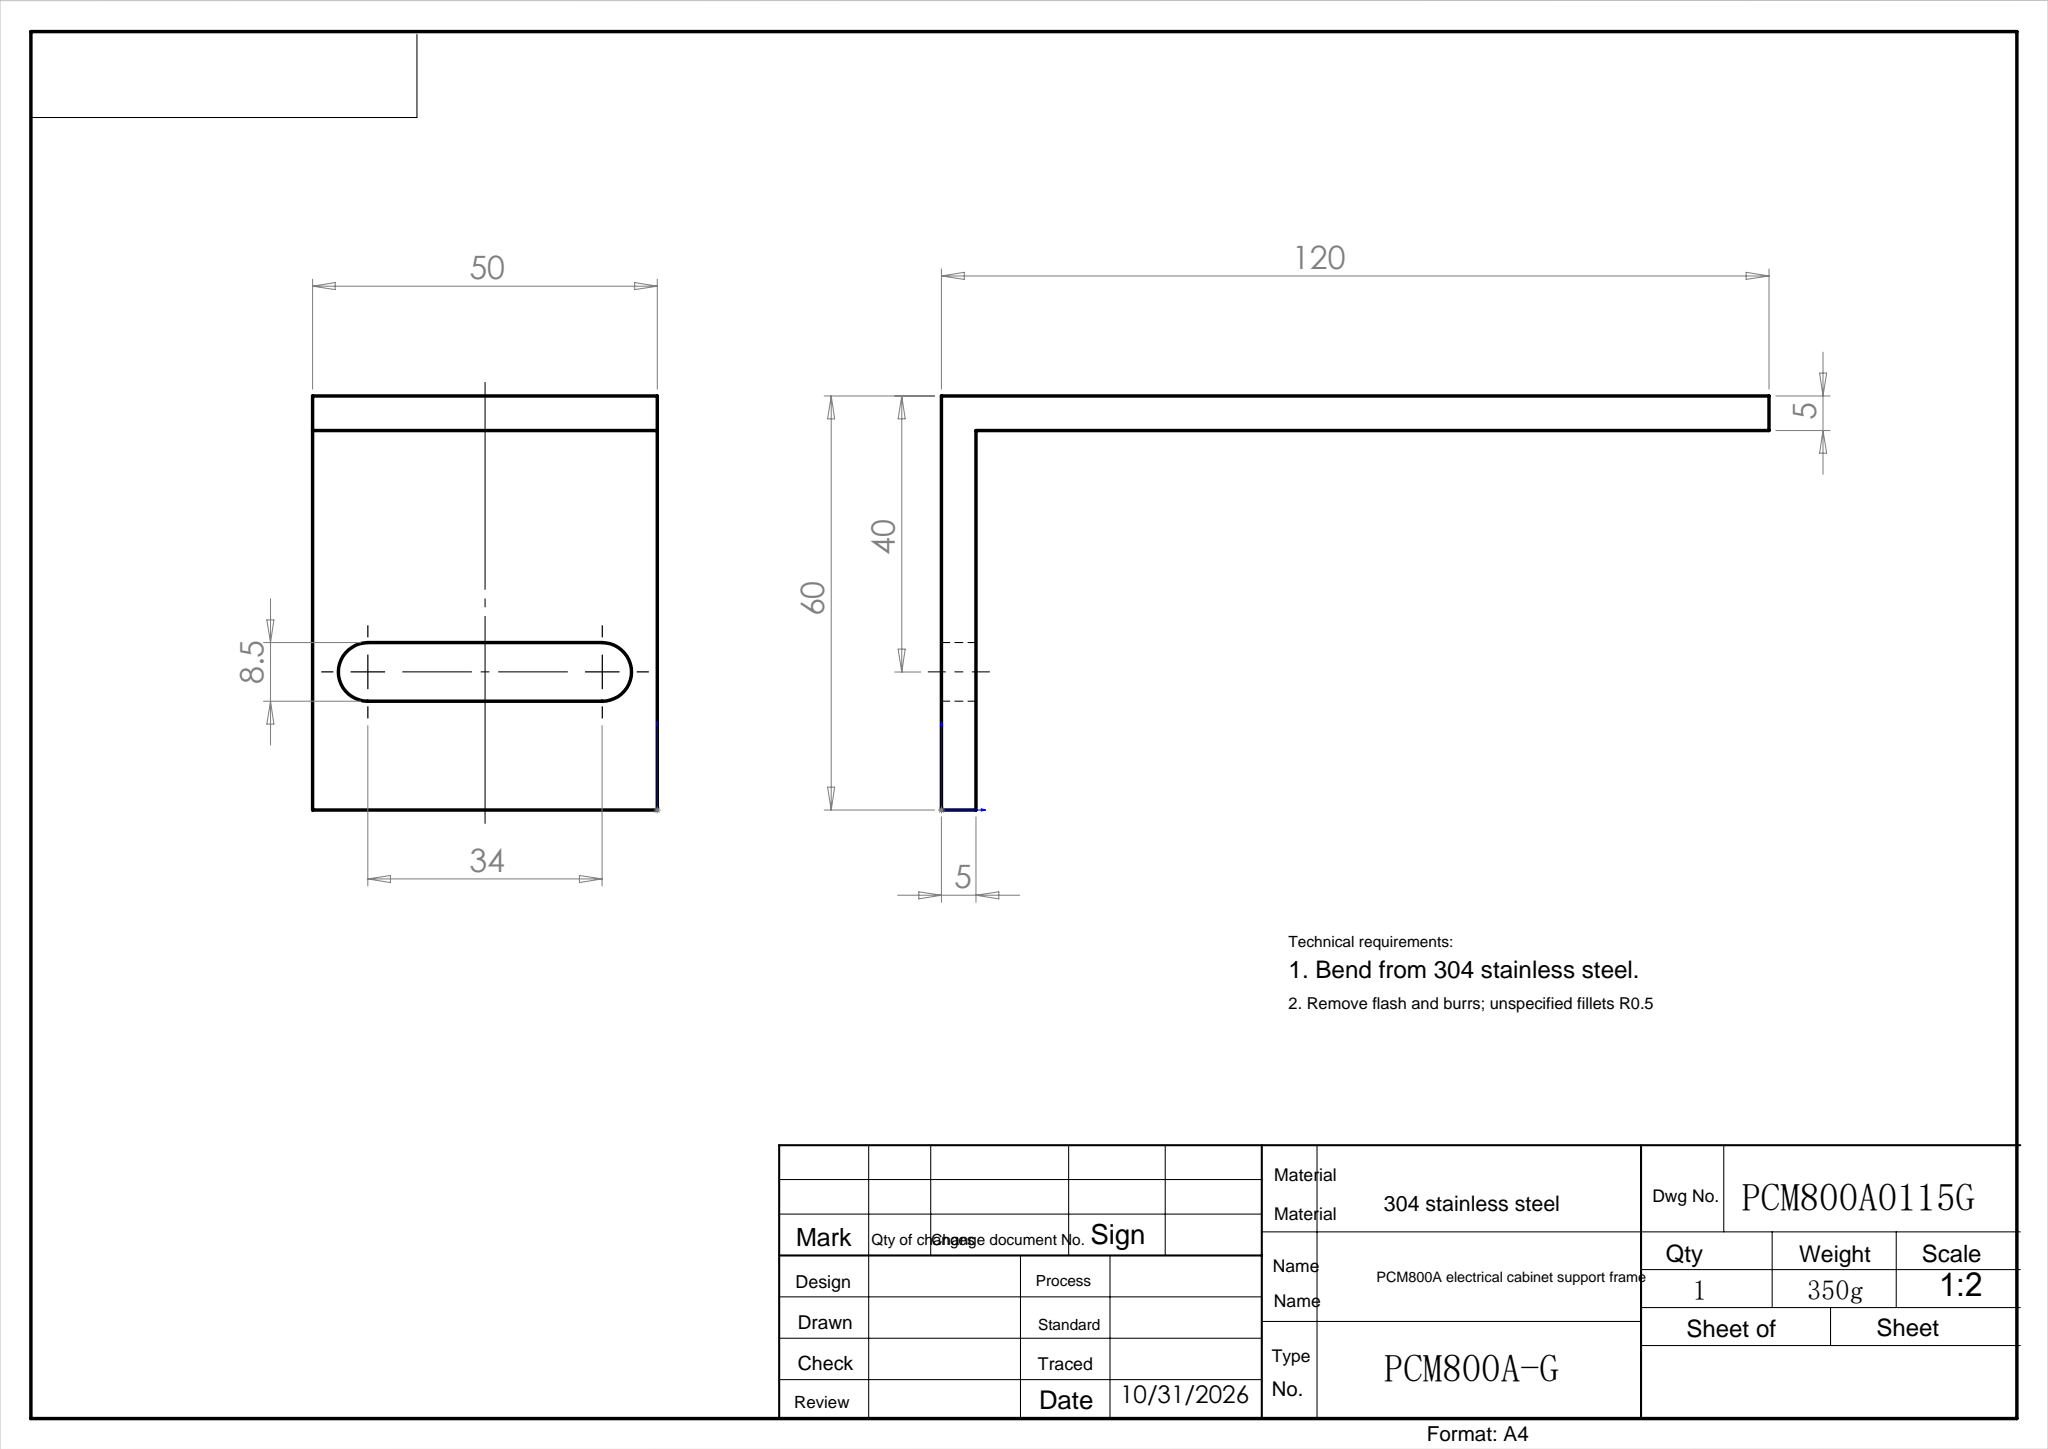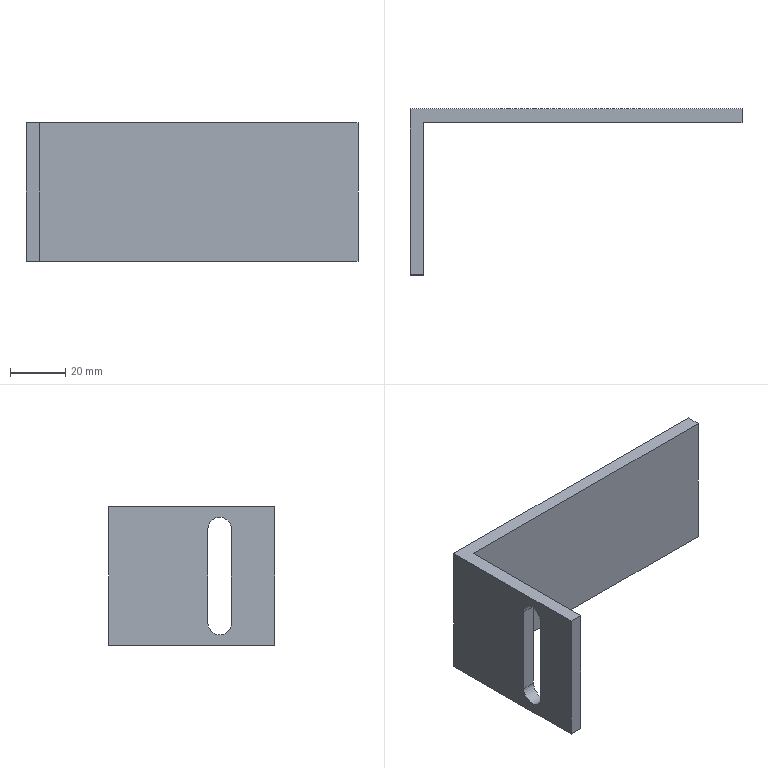Part | SolidWorks | features ExtruThin 1, ICE 1 | 1 solid | 13 faces | box 120 x 60 x 50 mm | volume 42021 mm3 | plane 10 | cylinder 3 | commonest cylinder face diameters 8.5 x3
STEP:
#1=CARTESIAN_POINT('',(5.,20.,46.25));
#2=VERTEX_POINT('',#1);
#3=CARTESIAN_POINT('',(5.,24.25,42.));
#4=VERTEX_POINT('',#3);
#5=CARTESIAN_POINT('',(5.,20.,42.));
#6=DIRECTION('',(-1.,0.,0.));
#7=DIRECTION('',(0.,0.,1.));
#8=AXIS2_PLACEMENT_3D('',#5,#6,#7);
#9=CIRCLE('',#8,4.25);
#10=EDGE_CURVE('',#2,#4,#9,.T.);
#11=ORIENTED_EDGE('',*,*,#10,.F.);
#12=CARTESIAN_POINT('',(0.,20.,46.25));
#13=VERTEX_POINT('',#12);
#14=CARTESIAN_POINT('',(10.,20.,46.25));
#15=DIRECTION('',(-1.,0.,0.));
#16=VECTOR('',#15,1000.);
#17=LINE('',#14,#16);
#18=EDGE_CURVE('',#2,#13,#17,.T.);
#19=ORIENTED_EDGE('',*,*,#18,.T.);
#20=CARTESIAN_POINT('',(0.,24.25,42.));
#21=VERTEX_POINT('',#20);
#22=CARTESIAN_POINT('',(0.,20.,42.));
#23=DIRECTION('',(-1.,0.,0.));
#24=DIRECTION('',(0.,0.,-1.));
#25=AXIS2_PLACEMENT_3D('',#22,#23,#24);
#26=CIRCLE('',#25,4.25);
#27=EDGE_CURVE('',#13,#21,#26,.T.);
#28=ORIENTED_EDGE('',*,*,#27,.T.);
#29=CARTESIAN_POINT('',(10.,24.25,42.));
#30=DIRECTION('',(-1.,0.,0.));
#31=VECTOR('',#30,1000.);
#32=LINE('',#29,#31);
#33=EDGE_CURVE('',#4,#21,#32,.T.);
#34=ORIENTED_EDGE('',*,*,#33,.F.);
#35=EDGE_LOOP('',(#11,#19,#28,#34));
#36=FACE_OUTER_BOUND('',#35,.T.);
#37=CARTESIAN_POINT('',(10.,20.,42.));
#38=DIRECTION('',(-1.,0.,0.));
#39=DIRECTION('',(0.,0.,1.));
#40=AXIS2_PLACEMENT_3D('',#37,#38,#39);
#41=CYLINDRICAL_SURFACE('',#40,4.25);
#42=ADVANCED_FACE('',(#36),#41,.F.);
#43=CARTESIAN_POINT('',(5.,55.,0.));
#44=VERTEX_POINT('',#43);
#45=CARTESIAN_POINT('',(120.,55.,0.));
#46=VERTEX_POINT('',#45);
#47=CARTESIAN_POINT('',(0.,55.,0.));
#48=DIRECTION('',(1.,0.,0.));
#49=VECTOR('',#48,1000.);
#50=LINE('',#47,#49);
#51=EDGE_CURVE('',#44,#46,#50,.T.);
#52=ORIENTED_EDGE('',*,*,#51,.T.);
#53=CARTESIAN_POINT('',(120.,55.,50.));
#54=VERTEX_POINT('',#53);
#55=CARTESIAN_POINT('',(120.,55.,50.));
#56=DIRECTION('',(0.,0.,-1.));
#57=VECTOR('',#56,1000.);
#58=LINE('',#55,#57);
#59=EDGE_CURVE('',#54,#46,#58,.T.);
#60=ORIENTED_EDGE('',*,*,#59,.F.);
#61=CARTESIAN_POINT('',(5.,55.,50.));
#62=VERTEX_POINT('',#61);
#63=CARTESIAN_POINT('',(0.,55.,50.));
#64=DIRECTION('',(1.,0.,0.));
#65=VECTOR('',#64,1000.);
#66=LINE('',#63,#65);
#67=EDGE_CURVE('',#62,#54,#66,.T.);
#68=ORIENTED_EDGE('',*,*,#67,.F.);
#69=CARTESIAN_POINT('',(5.,55.,50.));
#70=DIRECTION('',(0.,0.,-1.));
#71=VECTOR('',#70,1000.);
#72=LINE('',#69,#71);
#73=EDGE_CURVE('',#62,#44,#72,.T.);
#74=ORIENTED_EDGE('',*,*,#73,.T.);
#75=EDGE_LOOP('',(#52,#60,#68,#74));
#76=FACE_OUTER_BOUND('',#75,.T.);
#77=CARTESIAN_POINT('',(0.,55.,50.));
#78=DIRECTION('',(0.,1.,0.));
#79=DIRECTION('',(0.,0.,1.));
#80=AXIS2_PLACEMENT_3D('',#77,#78,#79);
#81=PLANE('',#80);
#82=ADVANCED_FACE('',(#76),#81,.F.);
#83=CARTESIAN_POINT('',(120.,60.,0.));
#84=VERTEX_POINT('',#83);
#85=CARTESIAN_POINT('',(120.,60.,0.));
#86=DIRECTION('',(0.,-1.,0.));
#87=VECTOR('',#86,1000.);
#88=LINE('',#85,#87);
#89=EDGE_CURVE('',#84,#46,#88,.T.);
#90=ORIENTED_EDGE('',*,*,#89,.F.);
#91=CARTESIAN_POINT('',(120.,60.,50.));
#92=VERTEX_POINT('',#91);
#93=CARTESIAN_POINT('',(120.,60.,50.));
#94=DIRECTION('',(0.,0.,-1.));
#95=VECTOR('',#94,1000.);
#96=LINE('',#93,#95);
#97=EDGE_CURVE('',#92,#84,#96,.T.);
#98=ORIENTED_EDGE('',*,*,#97,.F.);
#99=CARTESIAN_POINT('',(120.,60.,50.));
#100=DIRECTION('',(0.,-1.,0.));
#101=VECTOR('',#100,1000.);
#102=LINE('',#99,#101);
#103=EDGE_CURVE('',#92,#54,#102,.T.);
#104=ORIENTED_EDGE('',*,*,#103,.T.);
#105=ORIENTED_EDGE('',*,*,#59,.T.);
#106=EDGE_LOOP('',(#90,#98,#104,#105));
#107=FACE_OUTER_BOUND('',#106,.T.);
#108=CARTESIAN_POINT('',(120.,60.,50.));
#109=DIRECTION('',(1.,0.,0.));
#110=DIRECTION('',(0.,0.,-1.));
#111=AXIS2_PLACEMENT_3D('',#108,#109,#110);
#112=PLANE('',#111);
#113=ADVANCED_FACE('',(#107),#112,.T.);
#114=CARTESIAN_POINT('',(0.,60.,0.));
#115=VERTEX_POINT('',#114);
#116=CARTESIAN_POINT('',(0.,60.,0.));
#117=DIRECTION('',(1.,0.,0.));
#118=VECTOR('',#117,1000.);
#119=LINE('',#116,#118);
#120=EDGE_CURVE('',#115,#84,#119,.T.);
#121=ORIENTED_EDGE('',*,*,#120,.F.);
#122=CARTESIAN_POINT('',(0.,60.,50.));
#123=VERTEX_POINT('',#122);
#124=CARTESIAN_POINT('',(0.,60.,50.));
#125=DIRECTION('',(0.,0.,-1.));
#126=VECTOR('',#125,1000.);
#127=LINE('',#124,#126);
#128=EDGE_CURVE('',#123,#115,#127,.T.);
#129=ORIENTED_EDGE('',*,*,#128,.F.);
#130=CARTESIAN_POINT('',(0.,60.,50.));
#131=DIRECTION('',(1.,0.,0.));
#132=VECTOR('',#131,1000.);
#133=LINE('',#130,#132);
#134=EDGE_CURVE('',#123,#92,#133,.T.);
#135=ORIENTED_EDGE('',*,*,#134,.T.);
#136=ORIENTED_EDGE('',*,*,#97,.T.);
#137=EDGE_LOOP('',(#121,#129,#135,#136));
#138=FACE_OUTER_BOUND('',#137,.T.);
#139=CARTESIAN_POINT('',(0.,60.,50.));
#140=DIRECTION('',(0.,1.,0.));
#141=DIRECTION('',(0.,0.,1.));
#142=AXIS2_PLACEMENT_3D('',#139,#140,#141);
#143=PLANE('',#142);
#144=ADVANCED_FACE('',(#138),#143,.T.);
#145=CARTESIAN_POINT('',(0.,24.25,8.));
#146=VERTEX_POINT('',#145);
#147=CARTESIAN_POINT('',(0.,15.75,8.));
#148=VERTEX_POINT('',#147);
#149=CARTESIAN_POINT('',(0.,20.,8.));
#150=DIRECTION('',(-1.,0.,0.));
#151=DIRECTION('',(0.,0.,1.));
#152=AXIS2_PLACEMENT_3D('',#149,#150,#151);
#153=CIRCLE('',#152,4.25);
#154=EDGE_CURVE('',#146,#148,#153,.T.);
#155=ORIENTED_EDGE('',*,*,#154,.F.);
#156=CARTESIAN_POINT('',(0.,24.25,8.));
#157=DIRECTION('',(0.,0.,-1.));
#158=VECTOR('',#157,1000.);
#159=LINE('',#156,#158);
#160=EDGE_CURVE('',#21,#146,#159,.T.);
#161=ORIENTED_EDGE('',*,*,#160,.F.);
#162=ORIENTED_EDGE('',*,*,#27,.F.);
#163=CARTESIAN_POINT('',(0.,15.75,42.));
#164=VERTEX_POINT('',#163);
#165=CARTESIAN_POINT('',(0.,20.,42.));
#166=DIRECTION('',(-1.,0.,0.));
#167=DIRECTION('',(0.,0.,-1.));
#168=AXIS2_PLACEMENT_3D('',#165,#166,#167);
#169=CIRCLE('',#168,4.25);
#170=EDGE_CURVE('',#164,#13,#169,.T.);
#171=ORIENTED_EDGE('',*,*,#170,.F.);
#172=CARTESIAN_POINT('',(0.,15.75,8.));
#173=DIRECTION('',(0.,0.,1.));
#174=VECTOR('',#173,1000.);
#175=LINE('',#172,#174);
#176=EDGE_CURVE('',#148,#164,#175,.T.);
#177=ORIENTED_EDGE('',*,*,#176,.F.);
#178=EDGE_LOOP('',(#155,#161,#162,#171,#177));
#179=FACE_BOUND('',#178,.T.);
#180=CARTESIAN_POINT('',(0.,0.,0.));
#181=VERTEX_POINT('',#180);
#182=CARTESIAN_POINT('',(0.,0.,0.));
#183=DIRECTION('',(0.,1.,0.));
#184=VECTOR('',#183,1000.);
#185=LINE('',#182,#184);
#186=EDGE_CURVE('',#181,#115,#185,.T.);
#187=ORIENTED_EDGE('',*,*,#186,.F.);
#188=CARTESIAN_POINT('',(0.,0.,50.));
#189=VERTEX_POINT('',#188);
#190=CARTESIAN_POINT('',(0.,0.,50.));
#191=DIRECTION('',(0.,0.,-1.));
#192=VECTOR('',#191,1000.);
#193=LINE('',#190,#192);
#194=EDGE_CURVE('',#189,#181,#193,.T.);
#195=ORIENTED_EDGE('',*,*,#194,.F.);
#196=CARTESIAN_POINT('',(0.,0.,50.));
#197=DIRECTION('',(0.,1.,0.));
#198=VECTOR('',#197,1000.);
#199=LINE('',#196,#198);
#200=EDGE_CURVE('',#189,#123,#199,.T.);
#201=ORIENTED_EDGE('',*,*,#200,.T.);
#202=ORIENTED_EDGE('',*,*,#128,.T.);
#203=EDGE_LOOP('',(#187,#195,#201,#202));
#204=FACE_OUTER_BOUND('',#203,.T.);
#205=CARTESIAN_POINT('',(0.,0.,50.));
#206=DIRECTION('',(-1.,0.,0.));
#207=DIRECTION('',(0.,0.,1.));
#208=AXIS2_PLACEMENT_3D('',#205,#206,#207);
#209=PLANE('',#208);
#210=ADVANCED_FACE('',(#179,#204),#209,.T.);
#211=CARTESIAN_POINT('',(5.,0.,0.));
#212=VERTEX_POINT('',#211);
#213=CARTESIAN_POINT('',(5.,0.,0.));
#214=DIRECTION('',(-1.,0.,0.));
#215=VECTOR('',#214,1000.);
#216=LINE('',#213,#215);
#217=EDGE_CURVE('',#212,#181,#216,.T.);
#218=ORIENTED_EDGE('',*,*,#217,.F.);
#219=CARTESIAN_POINT('',(5.,0.,50.));
#220=VERTEX_POINT('',#219);
#221=CARTESIAN_POINT('',(5.,0.,50.));
#222=DIRECTION('',(0.,0.,-1.));
#223=VECTOR('',#222,1000.);
#224=LINE('',#221,#223);
#225=EDGE_CURVE('',#220,#212,#224,.T.);
#226=ORIENTED_EDGE('',*,*,#225,.F.);
#227=CARTESIAN_POINT('',(5.,0.,50.));
#228=DIRECTION('',(-1.,0.,0.));
#229=VECTOR('',#228,1000.);
#230=LINE('',#227,#229);
#231=EDGE_CURVE('',#220,#189,#230,.T.);
#232=ORIENTED_EDGE('',*,*,#231,.T.);
#233=ORIENTED_EDGE('',*,*,#194,.T.);
#234=EDGE_LOOP('',(#218,#226,#232,#233));
#235=FACE_OUTER_BOUND('',#234,.T.);
#236=CARTESIAN_POINT('',(5.,0.,50.));
#237=DIRECTION('',(0.,-1.,0.));
#238=DIRECTION('',(0.,0.,-1.));
#239=AXIS2_PLACEMENT_3D('',#236,#237,#238);
#240=PLANE('',#239);
#241=ADVANCED_FACE('',(#235),#240,.T.);
#242=CARTESIAN_POINT('',(5.,24.25,8.));
#243=VERTEX_POINT('',#242);
#244=CARTESIAN_POINT('',(5.,24.25,50.));
#245=DIRECTION('',(0.,0.,-1.));
#246=VECTOR('',#245,1000.);
#247=LINE('',#244,#246);
#248=EDGE_CURVE('',#4,#243,#247,.T.);
#249=ORIENTED_EDGE('',*,*,#248,.T.);
#250=CARTESIAN_POINT('',(5.,15.75,8.));
#251=VERTEX_POINT('',#250);
#252=CARTESIAN_POINT('',(5.,20.,8.));
#253=DIRECTION('',(-1.,0.,0.));
#254=DIRECTION('',(0.,0.,1.));
#255=AXIS2_PLACEMENT_3D('',#252,#253,#254);
#256=CIRCLE('',#255,4.25);
#257=EDGE_CURVE('',#243,#251,#256,.T.);
#258=ORIENTED_EDGE('',*,*,#257,.T.);
#259=CARTESIAN_POINT('',(5.,15.75,42.));
#260=VERTEX_POINT('',#259);
#261=CARTESIAN_POINT('',(5.,15.75,50.));
#262=DIRECTION('',(0.,0.,1.));
#263=VECTOR('',#262,1000.);
#264=LINE('',#261,#263);
#265=EDGE_CURVE('',#251,#260,#264,.T.);
#266=ORIENTED_EDGE('',*,*,#265,.T.);
#267=CARTESIAN_POINT('',(5.,20.,42.));
#268=DIRECTION('',(-1.,0.,0.));
#269=DIRECTION('',(0.,0.,1.));
#270=AXIS2_PLACEMENT_3D('',#267,#268,#269);
#271=CIRCLE('',#270,4.25);
#272=EDGE_CURVE('',#260,#2,#271,.T.);
#273=ORIENTED_EDGE('',*,*,#272,.T.);
#274=ORIENTED_EDGE('',*,*,#10,.T.);
#275=EDGE_LOOP('',(#249,#258,#266,#273,#274));
#276=FACE_BOUND('',#275,.T.);
#277=CARTESIAN_POINT('',(5.,0.,0.));
#278=DIRECTION('',(0.,1.,0.));
#279=VECTOR('',#278,1000.);
#280=LINE('',#277,#279);
#281=EDGE_CURVE('',#212,#44,#280,.T.);
#282=ORIENTED_EDGE('',*,*,#281,.T.);
#283=ORIENTED_EDGE('',*,*,#73,.F.);
#284=CARTESIAN_POINT('',(5.,0.,50.));
#285=DIRECTION('',(0.,1.,0.));
#286=VECTOR('',#285,1000.);
#287=LINE('',#284,#286);
#288=EDGE_CURVE('',#220,#62,#287,.T.);
#289=ORIENTED_EDGE('',*,*,#288,.F.);
#290=ORIENTED_EDGE('',*,*,#225,.T.);
#291=EDGE_LOOP('',(#282,#283,#289,#290));
#292=FACE_OUTER_BOUND('',#291,.T.);
#293=CARTESIAN_POINT('',(5.,0.,50.));
#294=DIRECTION('',(-1.,0.,0.));
#295=DIRECTION('',(0.,0.,1.));
#296=AXIS2_PLACEMENT_3D('',#293,#294,#295);
#297=PLANE('',#296);
#298=ADVANCED_FACE('',(#276,#292),#297,.F.);
#299=ORIENTED_EDGE('',*,*,#67,.T.);
#300=ORIENTED_EDGE('',*,*,#103,.F.);
#301=ORIENTED_EDGE('',*,*,#134,.F.);
#302=ORIENTED_EDGE('',*,*,#200,.F.);
#303=ORIENTED_EDGE('',*,*,#231,.F.);
#304=ORIENTED_EDGE('',*,*,#288,.T.);
#305=EDGE_LOOP('',(#299,#300,#301,#302,#303,#304));
#306=FACE_OUTER_BOUND('',#305,.T.);
#307=CARTESIAN_POINT('',(120.,55.,50.));
#308=DIRECTION('',(0.,0.,-1.));
#309=DIRECTION('',(-1.,0.,0.));
#310=AXIS2_PLACEMENT_3D('',#307,#308,#309);
#311=PLANE('',#310);
#312=ADVANCED_FACE('',(#306),#311,.F.);
#313=ORIENTED_EDGE('',*,*,#51,.F.);
#314=ORIENTED_EDGE('',*,*,#281,.F.);
#315=ORIENTED_EDGE('',*,*,#217,.T.);
#316=ORIENTED_EDGE('',*,*,#186,.T.);
#317=ORIENTED_EDGE('',*,*,#120,.T.);
#318=ORIENTED_EDGE('',*,*,#89,.T.);
#319=EDGE_LOOP('',(#313,#314,#315,#316,#317,#318));
#320=FACE_OUTER_BOUND('',#319,.T.);
#321=CARTESIAN_POINT('',(120.,55.,0.));
#322=DIRECTION('',(0.,0.,-1.));
#323=DIRECTION('',(-1.,0.,0.));
#324=AXIS2_PLACEMENT_3D('',#321,#322,#323);
#325=PLANE('',#324);
#326=ADVANCED_FACE('',(#320),#325,.T.);
#327=CARTESIAN_POINT('',(10.,24.25,8.));
#328=DIRECTION('',(-1.,0.,0.));
#329=VECTOR('',#328,1000.);
#330=LINE('',#327,#329);
#331=EDGE_CURVE('',#243,#146,#330,.T.);
#332=ORIENTED_EDGE('',*,*,#331,.T.);
#333=ORIENTED_EDGE('',*,*,#154,.T.);
#334=CARTESIAN_POINT('',(10.,15.75,8.));
#335=DIRECTION('',(-1.,0.,0.));
#336=VECTOR('',#335,1000.);
#337=LINE('',#334,#336);
#338=EDGE_CURVE('',#251,#148,#337,.T.);
#339=ORIENTED_EDGE('',*,*,#338,.F.);
#340=ORIENTED_EDGE('',*,*,#257,.F.);
#341=EDGE_LOOP('',(#332,#333,#339,#340));
#342=FACE_OUTER_BOUND('',#341,.T.);
#343=CARTESIAN_POINT('',(10.,20.,8.));
#344=DIRECTION('',(-1.,0.,0.));
#345=DIRECTION('',(0.,0.,1.));
#346=AXIS2_PLACEMENT_3D('',#343,#344,#345);
#347=CYLINDRICAL_SURFACE('',#346,4.25);
#348=ADVANCED_FACE('',(#342),#347,.F.);
#349=ORIENTED_EDGE('',*,*,#33,.T.);
#350=ORIENTED_EDGE('',*,*,#160,.T.);
#351=ORIENTED_EDGE('',*,*,#331,.F.);
#352=ORIENTED_EDGE('',*,*,#248,.F.);
#353=EDGE_LOOP('',(#349,#350,#351,#352));
#354=FACE_OUTER_BOUND('',#353,.T.);
#355=CARTESIAN_POINT('',(10.,24.25,8.));
#356=DIRECTION('',(0.,1.,0.));
#357=DIRECTION('',(0.,0.,1.));
#358=AXIS2_PLACEMENT_3D('',#355,#356,#357);
#359=PLANE('',#358);
#360=ADVANCED_FACE('',(#354),#359,.F.);
#361=ORIENTED_EDGE('',*,*,#18,.F.);
#362=ORIENTED_EDGE('',*,*,#272,.F.);
#363=CARTESIAN_POINT('',(10.,15.75,42.));
#364=DIRECTION('',(-1.,0.,0.));
#365=VECTOR('',#364,1000.);
#366=LINE('',#363,#365);
#367=EDGE_CURVE('',#260,#164,#366,.T.);
#368=ORIENTED_EDGE('',*,*,#367,.T.);
#369=ORIENTED_EDGE('',*,*,#170,.T.);
#370=EDGE_LOOP('',(#361,#362,#368,#369));
#371=FACE_OUTER_BOUND('',#370,.T.);
#372=CARTESIAN_POINT('',(10.,20.,42.));
#373=DIRECTION('',(-1.,0.,0.));
#374=DIRECTION('',(0.,0.,1.));
#375=AXIS2_PLACEMENT_3D('',#372,#373,#374);
#376=CYLINDRICAL_SURFACE('',#375,4.25);
#377=ADVANCED_FACE('',(#371),#376,.F.);
#378=ORIENTED_EDGE('',*,*,#338,.T.);
#379=ORIENTED_EDGE('',*,*,#176,.T.);
#380=ORIENTED_EDGE('',*,*,#367,.F.);
#381=ORIENTED_EDGE('',*,*,#265,.F.);
#382=EDGE_LOOP('',(#378,#379,#380,#381));
#383=FACE_OUTER_BOUND('',#382,.T.);
#384=CARTESIAN_POINT('',(10.,15.75,8.));
#385=DIRECTION('',(0.,-1.,0.));
#386=DIRECTION('',(0.,0.,-1.));
#387=AXIS2_PLACEMENT_3D('',#384,#385,#386);
#388=PLANE('',#387);
#389=ADVANCED_FACE('',(#383),#388,.F.);
#390=CLOSED_SHELL('',(#42,#82,#113,#144,#210,#241,#298,#312,#326,#348,#360,#377,#389));
#391=MANIFOLD_SOLID_BREP('',#390);
#392=CARTESIAN_POINT('',(0.,0.,0.));
#393=DIRECTION('',(0.,0.,1.));
#394=DIRECTION('',(1.,0.,0.));
#395=AXIS2_PLACEMENT_3D('',#392,#393,#394);
#396=(LENGTH_UNIT()NAMED_UNIT(*)SI_UNIT(.MILLI.,.METRE.));
#397=UNCERTAINTY_MEASURE_WITH_UNIT(LENGTH_MEASURE(0.00001),#396,'','');
#398=(NAMED_UNIT(*)PLANE_ANGLE_UNIT()SI_UNIT($,.RADIAN.));
#399=(NAMED_UNIT(*)SI_UNIT($,.STERADIAN.)SOLID_ANGLE_UNIT());
#400=(GEOMETRIC_REPRESENTATION_CONTEXT(3)GLOBAL_UNCERTAINTY_ASSIGNED_CONTEXT((#397))GLOBAL_UNIT_ASSIGNED_CONTEXT((#396,#398,#399))REPRESENTATION_CONTEXT('',''));
#401=ADVANCED_BREP_SHAPE_REPRESENTATION('',(#391,#395),#400);